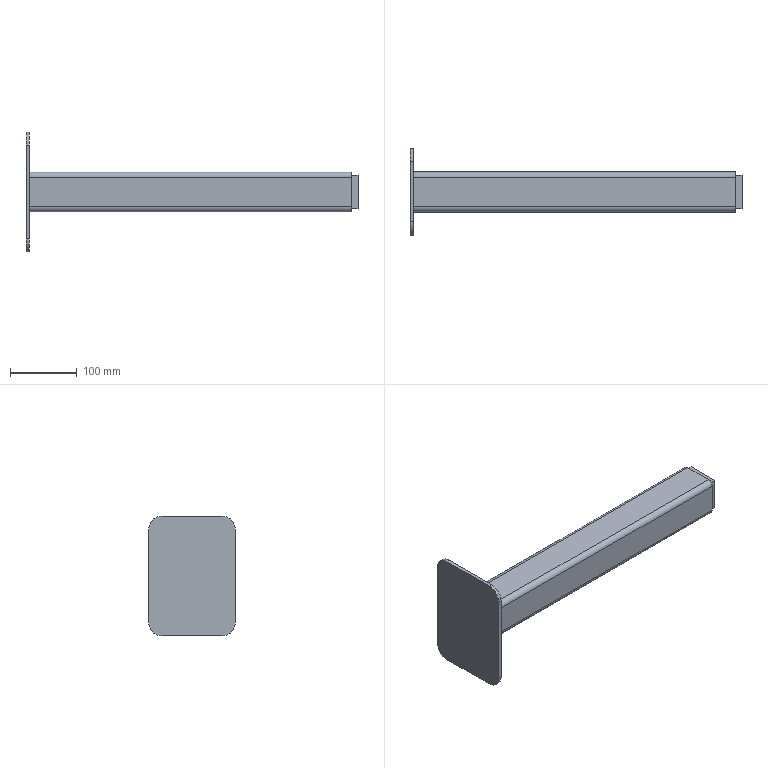Part | SolidWorks | features ICE 2, HoleWzd 1, WeldMemberFeat 1, WeldmentFeature 1 | 3 solids | 36 faces | box 498.5 x 130 x 180 mm | volume 585064 mm3 | plane 22 | cylinder 14 | commonest cylinder face diameters 8 x4 16 x4 40 x4 17.5 x2
STEP:
#1=CARTESIAN_POINT('',(0.,30.,22.));
#2=VERTEX_POINT('',#1);
#3=CARTESIAN_POINT('',(0.,22.,30.));
#4=VERTEX_POINT('',#3);
#5=CARTESIAN_POINT('',(0.,22.,22.));
#6=DIRECTION('',(1.,0.,0.));
#7=DIRECTION('',(0.,0.,-1.));
#8=AXIS2_PLACEMENT_3D('',#5,#6,#7);
#9=CIRCLE('',#8,8.);
#10=EDGE_CURVE('',#2,#4,#9,.T.);
#11=ORIENTED_EDGE('',*,*,#10,.T.);
#12=CARTESIAN_POINT('',(483.5,22.,30.));
#13=VERTEX_POINT('',#12);
#14=CARTESIAN_POINT('',(483.5,22.,30.));
#15=DIRECTION('',(-1.,0.,0.));
#16=VECTOR('',#15,1000.);
#17=LINE('',#14,#16);
#18=EDGE_CURVE('',#13,#4,#17,.T.);
#19=ORIENTED_EDGE('',*,*,#18,.F.);
#20=CARTESIAN_POINT('',(483.5,30.,22.));
#21=VERTEX_POINT('',#20);
#22=CARTESIAN_POINT('',(483.5,22.,22.));
#23=DIRECTION('',(1.,0.,0.));
#24=DIRECTION('',(0.,0.,-1.));
#25=AXIS2_PLACEMENT_3D('',#22,#23,#24);
#26=CIRCLE('',#25,8.);
#27=EDGE_CURVE('',#21,#13,#26,.T.);
#28=ORIENTED_EDGE('',*,*,#27,.F.);
#29=CARTESIAN_POINT('',(483.5,30.,22.));
#30=DIRECTION('',(-1.,0.,0.));
#31=VECTOR('',#30,1000.);
#32=LINE('',#29,#31);
#33=EDGE_CURVE('',#21,#2,#32,.T.);
#34=ORIENTED_EDGE('',*,*,#33,.T.);
#35=EDGE_LOOP('',(#11,#19,#28,#34));
#36=FACE_OUTER_BOUND('',#35,.T.);
#37=CARTESIAN_POINT('',(483.5,22.,22.));
#38=DIRECTION('',(-1.,0.,0.));
#39=DIRECTION('',(0.,0.,1.));
#40=AXIS2_PLACEMENT_3D('',#37,#38,#39);
#41=CYLINDRICAL_SURFACE('',#40,8.);
#42=ADVANCED_FACE('',(#36),#41,.T.);
#43=CARTESIAN_POINT('',(0.,-22.,30.));
#44=VERTEX_POINT('',#43);
#45=CARTESIAN_POINT('',(0.,22.,30.));
#46=DIRECTION('',(0.,-1.,0.));
#47=VECTOR('',#46,1000.);
#48=LINE('',#45,#47);
#49=EDGE_CURVE('',#4,#44,#48,.T.);
#50=ORIENTED_EDGE('',*,*,#49,.T.);
#51=CARTESIAN_POINT('',(483.5,-22.,30.));
#52=VERTEX_POINT('',#51);
#53=CARTESIAN_POINT('',(483.5,-22.,30.));
#54=DIRECTION('',(-1.,0.,0.));
#55=VECTOR('',#54,1000.);
#56=LINE('',#53,#55);
#57=EDGE_CURVE('',#52,#44,#56,.T.);
#58=ORIENTED_EDGE('',*,*,#57,.F.);
#59=CARTESIAN_POINT('',(483.5,22.,30.));
#60=DIRECTION('',(0.,-1.,0.));
#61=VECTOR('',#60,1000.);
#62=LINE('',#59,#61);
#63=EDGE_CURVE('',#13,#52,#62,.T.);
#64=ORIENTED_EDGE('',*,*,#63,.F.);
#65=ORIENTED_EDGE('',*,*,#18,.T.);
#66=EDGE_LOOP('',(#50,#58,#64,#65));
#67=FACE_OUTER_BOUND('',#66,.T.);
#68=CARTESIAN_POINT('',(483.5,22.,30.));
#69=DIRECTION('',(0.,0.,-1.));
#70=DIRECTION('',(-1.,0.,0.));
#71=AXIS2_PLACEMENT_3D('',#68,#69,#70);
#72=PLANE('',#71);
#73=ADVANCED_FACE('',(#67),#72,.F.);
#74=CARTESIAN_POINT('',(0.,-30.,22.));
#75=VERTEX_POINT('',#74);
#76=CARTESIAN_POINT('',(0.,-22.,22.));
#77=DIRECTION('',(1.,0.,0.));
#78=DIRECTION('',(0.,0.,-1.));
#79=AXIS2_PLACEMENT_3D('',#76,#77,#78);
#80=CIRCLE('',#79,8.);
#81=EDGE_CURVE('',#44,#75,#80,.T.);
#82=ORIENTED_EDGE('',*,*,#81,.T.);
#83=CARTESIAN_POINT('',(483.5,-30.,22.));
#84=VERTEX_POINT('',#83);
#85=CARTESIAN_POINT('',(483.5,-30.,22.));
#86=DIRECTION('',(-1.,0.,0.));
#87=VECTOR('',#86,1000.);
#88=LINE('',#85,#87);
#89=EDGE_CURVE('',#84,#75,#88,.T.);
#90=ORIENTED_EDGE('',*,*,#89,.F.);
#91=CARTESIAN_POINT('',(483.5,-22.,22.));
#92=DIRECTION('',(1.,0.,0.));
#93=DIRECTION('',(0.,0.,-1.));
#94=AXIS2_PLACEMENT_3D('',#91,#92,#93);
#95=CIRCLE('',#94,8.);
#96=EDGE_CURVE('',#52,#84,#95,.T.);
#97=ORIENTED_EDGE('',*,*,#96,.F.);
#98=ORIENTED_EDGE('',*,*,#57,.T.);
#99=EDGE_LOOP('',(#82,#90,#97,#98));
#100=FACE_OUTER_BOUND('',#99,.T.);
#101=CARTESIAN_POINT('',(483.5,-22.,22.));
#102=DIRECTION('',(-1.,0.,0.));
#103=DIRECTION('',(0.,0.,1.));
#104=AXIS2_PLACEMENT_3D('',#101,#102,#103);
#105=CYLINDRICAL_SURFACE('',#104,8.);
#106=ADVANCED_FACE('',(#100),#105,.T.);
#107=CARTESIAN_POINT('',(0.,-30.,-22.));
#108=VERTEX_POINT('',#107);
#109=CARTESIAN_POINT('',(0.,-30.,-22.));
#110=DIRECTION('',(0.,0.,-1.));
#111=VECTOR('',#110,1000.);
#112=LINE('',#109,#111);
#113=EDGE_CURVE('',#75,#108,#112,.T.);
#114=ORIENTED_EDGE('',*,*,#113,.T.);
#115=CARTESIAN_POINT('',(483.5,-30.,-22.));
#116=VERTEX_POINT('',#115);
#117=CARTESIAN_POINT('',(483.5,-30.,-22.));
#118=DIRECTION('',(-1.,0.,0.));
#119=VECTOR('',#118,1000.);
#120=LINE('',#117,#119);
#121=EDGE_CURVE('',#116,#108,#120,.T.);
#122=ORIENTED_EDGE('',*,*,#121,.F.);
#123=CARTESIAN_POINT('',(483.5,-30.,-22.));
#124=DIRECTION('',(0.,0.,-1.));
#125=VECTOR('',#124,1000.);
#126=LINE('',#123,#125);
#127=EDGE_CURVE('',#84,#116,#126,.T.);
#128=ORIENTED_EDGE('',*,*,#127,.F.);
#129=ORIENTED_EDGE('',*,*,#89,.T.);
#130=EDGE_LOOP('',(#114,#122,#128,#129));
#131=FACE_OUTER_BOUND('',#130,.T.);
#132=CARTESIAN_POINT('',(483.5,-30.,-22.));
#133=DIRECTION('',(0.,1.,0.));
#134=DIRECTION('',(0.,0.,1.));
#135=AXIS2_PLACEMENT_3D('',#132,#133,#134);
#136=PLANE('',#135);
#137=ADVANCED_FACE('',(#131),#136,.F.);
#138=CARTESIAN_POINT('',(0.,-22.,-30.));
#139=VERTEX_POINT('',#138);
#140=CARTESIAN_POINT('',(0.,-22.,-22.));
#141=DIRECTION('',(1.,0.,0.));
#142=DIRECTION('',(0.,0.,-1.));
#143=AXIS2_PLACEMENT_3D('',#140,#141,#142);
#144=CIRCLE('',#143,8.);
#145=EDGE_CURVE('',#108,#139,#144,.T.);
#146=ORIENTED_EDGE('',*,*,#145,.T.);
#147=CARTESIAN_POINT('',(483.5,-22.,-30.));
#148=VERTEX_POINT('',#147);
#149=CARTESIAN_POINT('',(483.5,-22.,-30.));
#150=DIRECTION('',(-1.,0.,0.));
#151=VECTOR('',#150,1000.);
#152=LINE('',#149,#151);
#153=EDGE_CURVE('',#148,#139,#152,.T.);
#154=ORIENTED_EDGE('',*,*,#153,.F.);
#155=CARTESIAN_POINT('',(483.5,-22.,-22.));
#156=DIRECTION('',(1.,0.,0.));
#157=DIRECTION('',(0.,0.,-1.));
#158=AXIS2_PLACEMENT_3D('',#155,#156,#157);
#159=CIRCLE('',#158,8.);
#160=EDGE_CURVE('',#116,#148,#159,.T.);
#161=ORIENTED_EDGE('',*,*,#160,.F.);
#162=ORIENTED_EDGE('',*,*,#121,.T.);
#163=EDGE_LOOP('',(#146,#154,#161,#162));
#164=FACE_OUTER_BOUND('',#163,.T.);
#165=CARTESIAN_POINT('',(483.5,-22.,-22.));
#166=DIRECTION('',(-1.,0.,0.));
#167=DIRECTION('',(0.,0.,1.));
#168=AXIS2_PLACEMENT_3D('',#165,#166,#167);
#169=CYLINDRICAL_SURFACE('',#168,8.);
#170=ADVANCED_FACE('',(#164),#169,.T.);
#171=CARTESIAN_POINT('',(0.,22.,-30.));
#172=VERTEX_POINT('',#171);
#173=CARTESIAN_POINT('',(0.,-22.,-30.));
#174=DIRECTION('',(0.,1.,0.));
#175=VECTOR('',#174,1000.);
#176=LINE('',#173,#175);
#177=EDGE_CURVE('',#139,#172,#176,.T.);
#178=ORIENTED_EDGE('',*,*,#177,.T.);
#179=CARTESIAN_POINT('',(483.5,22.,-30.));
#180=VERTEX_POINT('',#179);
#181=CARTESIAN_POINT('',(483.5,22.,-30.));
#182=DIRECTION('',(-1.,0.,0.));
#183=VECTOR('',#182,1000.);
#184=LINE('',#181,#183);
#185=EDGE_CURVE('',#180,#172,#184,.T.);
#186=ORIENTED_EDGE('',*,*,#185,.F.);
#187=CARTESIAN_POINT('',(483.5,-22.,-30.));
#188=DIRECTION('',(0.,1.,0.));
#189=VECTOR('',#188,1000.);
#190=LINE('',#187,#189);
#191=EDGE_CURVE('',#148,#180,#190,.T.);
#192=ORIENTED_EDGE('',*,*,#191,.F.);
#193=ORIENTED_EDGE('',*,*,#153,.T.);
#194=EDGE_LOOP('',(#178,#186,#192,#193));
#195=FACE_OUTER_BOUND('',#194,.T.);
#196=CARTESIAN_POINT('',(483.5,-22.,-30.));
#197=DIRECTION('',(0.,0.,1.));
#198=DIRECTION('',(1.,0.,0.));
#199=AXIS2_PLACEMENT_3D('',#196,#197,#198);
#200=PLANE('',#199);
#201=ADVANCED_FACE('',(#195),#200,.F.);
#202=CARTESIAN_POINT('',(0.,30.,-22.));
#203=VERTEX_POINT('',#202);
#204=CARTESIAN_POINT('',(0.,22.,-22.));
#205=DIRECTION('',(1.,0.,0.));
#206=DIRECTION('',(0.,0.,-1.));
#207=AXIS2_PLACEMENT_3D('',#204,#205,#206);
#208=CIRCLE('',#207,8.);
#209=EDGE_CURVE('',#172,#203,#208,.T.);
#210=ORIENTED_EDGE('',*,*,#209,.T.);
#211=CARTESIAN_POINT('',(483.5,30.,-22.));
#212=VERTEX_POINT('',#211);
#213=CARTESIAN_POINT('',(483.5,30.,-22.));
#214=DIRECTION('',(-1.,0.,0.));
#215=VECTOR('',#214,1000.);
#216=LINE('',#213,#215);
#217=EDGE_CURVE('',#212,#203,#216,.T.);
#218=ORIENTED_EDGE('',*,*,#217,.F.);
#219=CARTESIAN_POINT('',(483.5,22.,-22.));
#220=DIRECTION('',(1.,0.,0.));
#221=DIRECTION('',(0.,0.,-1.));
#222=AXIS2_PLACEMENT_3D('',#219,#220,#221);
#223=CIRCLE('',#222,8.);
#224=EDGE_CURVE('',#180,#212,#223,.T.);
#225=ORIENTED_EDGE('',*,*,#224,.F.);
#226=ORIENTED_EDGE('',*,*,#185,.T.);
#227=EDGE_LOOP('',(#210,#218,#225,#226));
#228=FACE_OUTER_BOUND('',#227,.T.);
#229=CARTESIAN_POINT('',(483.5,22.,-22.));
#230=DIRECTION('',(-1.,0.,0.));
#231=DIRECTION('',(0.,0.,1.));
#232=AXIS2_PLACEMENT_3D('',#229,#230,#231);
#233=CYLINDRICAL_SURFACE('',#232,8.);
#234=ADVANCED_FACE('',(#228),#233,.T.);
#235=CARTESIAN_POINT('',(0.,-22.,26.));
#236=VERTEX_POINT('',#235);
#237=CARTESIAN_POINT('',(0.,-26.,22.));
#238=VERTEX_POINT('',#237);
#239=CARTESIAN_POINT('',(0.,-22.,22.));
#240=DIRECTION('',(1.,0.,0.));
#241=DIRECTION('',(0.,0.,-1.));
#242=AXIS2_PLACEMENT_3D('',#239,#240,#241);
#243=CIRCLE('',#242,4.);
#244=EDGE_CURVE('',#236,#238,#243,.T.);
#245=ORIENTED_EDGE('',*,*,#244,.F.);
#246=CARTESIAN_POINT('',(483.5,-22.,26.));
#247=VERTEX_POINT('',#246);
#248=CARTESIAN_POINT('',(483.5,-22.,26.));
#249=DIRECTION('',(-1.,0.,0.));
#250=VECTOR('',#249,1000.);
#251=LINE('',#248,#250);
#252=EDGE_CURVE('',#247,#236,#251,.T.);
#253=ORIENTED_EDGE('',*,*,#252,.F.);
#254=CARTESIAN_POINT('',(483.5,-26.,22.));
#255=VERTEX_POINT('',#254);
#256=CARTESIAN_POINT('',(483.5,-22.,22.));
#257=DIRECTION('',(1.,0.,0.));
#258=DIRECTION('',(0.,0.,-1.));
#259=AXIS2_PLACEMENT_3D('',#256,#257,#258);
#260=CIRCLE('',#259,4.);
#261=EDGE_CURVE('',#247,#255,#260,.T.);
#262=ORIENTED_EDGE('',*,*,#261,.T.);
#263=CARTESIAN_POINT('',(483.5,-26.,22.));
#264=DIRECTION('',(-1.,0.,0.));
#265=VECTOR('',#264,1000.);
#266=LINE('',#263,#265);
#267=EDGE_CURVE('',#255,#238,#266,.T.);
#268=ORIENTED_EDGE('',*,*,#267,.T.);
#269=EDGE_LOOP('',(#245,#253,#262,#268));
#270=FACE_OUTER_BOUND('',#269,.T.);
#271=CARTESIAN_POINT('',(483.5,-22.,22.));
#272=DIRECTION('',(-1.,0.,0.));
#273=DIRECTION('',(0.,0.,1.));
#274=AXIS2_PLACEMENT_3D('',#271,#272,#273);
#275=CYLINDRICAL_SURFACE('',#274,4.);
#276=ADVANCED_FACE('',(#270),#275,.F.);
#277=CARTESIAN_POINT('',(0.,22.,26.));
#278=VERTEX_POINT('',#277);
#279=CARTESIAN_POINT('',(0.,22.,26.));
#280=DIRECTION('',(0.,-1.,0.));
#281=VECTOR('',#280,1000.);
#282=LINE('',#279,#281);
#283=EDGE_CURVE('',#278,#236,#282,.T.);
#284=ORIENTED_EDGE('',*,*,#283,.F.);
#285=CARTESIAN_POINT('',(483.5,22.,26.));
#286=VERTEX_POINT('',#285);
#287=CARTESIAN_POINT('',(483.5,22.,26.));
#288=DIRECTION('',(-1.,0.,0.));
#289=VECTOR('',#288,1000.);
#290=LINE('',#287,#289);
#291=EDGE_CURVE('',#286,#278,#290,.T.);
#292=ORIENTED_EDGE('',*,*,#291,.F.);
#293=CARTESIAN_POINT('',(483.5,22.,26.));
#294=DIRECTION('',(0.,-1.,0.));
#295=VECTOR('',#294,1000.);
#296=LINE('',#293,#295);
#297=EDGE_CURVE('',#286,#247,#296,.T.);
#298=ORIENTED_EDGE('',*,*,#297,.T.);
#299=ORIENTED_EDGE('',*,*,#252,.T.);
#300=EDGE_LOOP('',(#284,#292,#298,#299));
#301=FACE_OUTER_BOUND('',#300,.T.);
#302=CARTESIAN_POINT('',(483.5,22.,26.));
#303=DIRECTION('',(0.,0.,-1.));
#304=DIRECTION('',(-1.,0.,0.));
#305=AXIS2_PLACEMENT_3D('',#302,#303,#304);
#306=PLANE('',#305);
#307=ADVANCED_FACE('',(#301),#306,.T.);
#308=CARTESIAN_POINT('',(0.,26.,22.));
#309=VERTEX_POINT('',#308);
#310=CARTESIAN_POINT('',(0.,22.,22.));
#311=DIRECTION('',(1.,0.,0.));
#312=DIRECTION('',(0.,0.,-1.));
#313=AXIS2_PLACEMENT_3D('',#310,#311,#312);
#314=CIRCLE('',#313,4.);
#315=EDGE_CURVE('',#309,#278,#314,.T.);
#316=ORIENTED_EDGE('',*,*,#315,.F.);
#317=CARTESIAN_POINT('',(483.5,26.,22.));
#318=VERTEX_POINT('',#317);
#319=CARTESIAN_POINT('',(483.5,26.,22.));
#320=DIRECTION('',(-1.,0.,0.));
#321=VECTOR('',#320,1000.);
#322=LINE('',#319,#321);
#323=EDGE_CURVE('',#318,#309,#322,.T.);
#324=ORIENTED_EDGE('',*,*,#323,.F.);
#325=CARTESIAN_POINT('',(483.5,22.,22.));
#326=DIRECTION('',(1.,0.,0.));
#327=DIRECTION('',(0.,0.,-1.));
#328=AXIS2_PLACEMENT_3D('',#325,#326,#327);
#329=CIRCLE('',#328,4.);
#330=EDGE_CURVE('',#318,#286,#329,.T.);
#331=ORIENTED_EDGE('',*,*,#330,.T.);
#332=ORIENTED_EDGE('',*,*,#291,.T.);
#333=EDGE_LOOP('',(#316,#324,#331,#332));
#334=FACE_OUTER_BOUND('',#333,.T.);
#335=CARTESIAN_POINT('',(483.5,22.,22.));
#336=DIRECTION('',(-1.,0.,0.));
#337=DIRECTION('',(0.,0.,1.));
#338=AXIS2_PLACEMENT_3D('',#335,#336,#337);
#339=CYLINDRICAL_SURFACE('',#338,4.);
#340=ADVANCED_FACE('',(#334),#339,.F.);
#341=CARTESIAN_POINT('',(0.,26.,-22.));
#342=VERTEX_POINT('',#341);
#343=CARTESIAN_POINT('',(0.,26.,22.));
#344=DIRECTION('',(0.,0.,1.));
#345=VECTOR('',#344,1000.);
#346=LINE('',#343,#345);
#347=EDGE_CURVE('',#342,#309,#346,.T.);
#348=ORIENTED_EDGE('',*,*,#347,.F.);
#349=CARTESIAN_POINT('',(483.5,26.,-22.));
#350=VERTEX_POINT('',#349);
#351=CARTESIAN_POINT('',(483.5,26.,-22.));
#352=DIRECTION('',(-1.,0.,0.));
#353=VECTOR('',#352,1000.);
#354=LINE('',#351,#353);
#355=EDGE_CURVE('',#350,#342,#354,.T.);
#356=ORIENTED_EDGE('',*,*,#355,.F.);
#357=CARTESIAN_POINT('',(483.5,26.,22.));
#358=DIRECTION('',(0.,0.,1.));
#359=VECTOR('',#358,1000.);
#360=LINE('',#357,#359);
#361=EDGE_CURVE('',#350,#318,#360,.T.);
#362=ORIENTED_EDGE('',*,*,#361,.T.);
#363=ORIENTED_EDGE('',*,*,#323,.T.);
#364=EDGE_LOOP('',(#348,#356,#362,#363));
#365=FACE_OUTER_BOUND('',#364,.T.);
#366=CARTESIAN_POINT('',(483.5,26.,22.));
#367=DIRECTION('',(0.,-1.,0.));
#368=DIRECTION('',(0.,0.,-1.));
#369=AXIS2_PLACEMENT_3D('',#366,#367,#368);
#370=PLANE('',#369);
#371=ADVANCED_FACE('',(#365),#370,.T.);
#372=CARTESIAN_POINT('',(0.,22.,-26.));
#373=VERTEX_POINT('',#372);
#374=CARTESIAN_POINT('',(0.,22.,-22.));
#375=DIRECTION('',(1.,0.,0.));
#376=DIRECTION('',(0.,0.,-1.));
#377=AXIS2_PLACEMENT_3D('',#374,#375,#376);
#378=CIRCLE('',#377,4.);
#379=EDGE_CURVE('',#373,#342,#378,.T.);
#380=ORIENTED_EDGE('',*,*,#379,.F.);
#381=CARTESIAN_POINT('',(483.5,22.,-26.));
#382=VERTEX_POINT('',#381);
#383=CARTESIAN_POINT('',(483.5,22.,-26.));
#384=DIRECTION('',(-1.,0.,0.));
#385=VECTOR('',#384,1000.);
#386=LINE('',#383,#385);
#387=EDGE_CURVE('',#382,#373,#386,.T.);
#388=ORIENTED_EDGE('',*,*,#387,.F.);
#389=CARTESIAN_POINT('',(483.5,22.,-22.));
#390=DIRECTION('',(1.,0.,0.));
#391=DIRECTION('',(0.,0.,-1.));
#392=AXIS2_PLACEMENT_3D('',#389,#390,#391);
#393=CIRCLE('',#392,4.);
#394=EDGE_CURVE('',#382,#350,#393,.T.);
#395=ORIENTED_EDGE('',*,*,#394,.T.);
#396=ORIENTED_EDGE('',*,*,#355,.T.);
#397=EDGE_LOOP('',(#380,#388,#395,#396));
#398=FACE_OUTER_BOUND('',#397,.T.);
#399=CARTESIAN_POINT('',(483.5,22.,-22.));
#400=DIRECTION('',(-1.,0.,0.));
#401=DIRECTION('',(0.,0.,1.));
#402=AXIS2_PLACEMENT_3D('',#399,#400,#401);
#403=CYLINDRICAL_SURFACE('',#402,4.);
#404=ADVANCED_FACE('',(#398),#403,.F.);
#405=CARTESIAN_POINT('',(0.,-22.,-26.));
#406=VERTEX_POINT('',#405);
#407=CARTESIAN_POINT('',(0.,-22.,-26.));
#408=DIRECTION('',(0.,1.,0.));
#409=VECTOR('',#408,1000.);
#410=LINE('',#407,#409);
#411=EDGE_CURVE('',#406,#373,#410,.T.);
#412=ORIENTED_EDGE('',*,*,#411,.F.);
#413=CARTESIAN_POINT('',(483.5,-22.,-26.));
#414=VERTEX_POINT('',#413);
#415=CARTESIAN_POINT('',(483.5,-22.,-26.));
#416=DIRECTION('',(-1.,0.,0.));
#417=VECTOR('',#416,1000.);
#418=LINE('',#415,#417);
#419=EDGE_CURVE('',#414,#406,#418,.T.);
#420=ORIENTED_EDGE('',*,*,#419,.F.);
#421=CARTESIAN_POINT('',(483.5,-22.,-26.));
#422=DIRECTION('',(0.,1.,0.));
#423=VECTOR('',#422,1000.);
#424=LINE('',#421,#423);
#425=EDGE_CURVE('',#414,#382,#424,.T.);
#426=ORIENTED_EDGE('',*,*,#425,.T.);
#427=ORIENTED_EDGE('',*,*,#387,.T.);
#428=EDGE_LOOP('',(#412,#420,#426,#427));
#429=FACE_OUTER_BOUND('',#428,.T.);
#430=CARTESIAN_POINT('',(483.5,-22.,-26.));
#431=DIRECTION('',(0.,0.,1.));
#432=DIRECTION('',(1.,0.,0.));
#433=AXIS2_PLACEMENT_3D('',#430,#431,#432);
#434=PLANE('',#433);
#435=ADVANCED_FACE('',(#429),#434,.T.);
#436=CARTESIAN_POINT('',(0.,-26.,-22.));
#437=VERTEX_POINT('',#436);
#438=CARTESIAN_POINT('',(0.,-22.,-22.));
#439=DIRECTION('',(1.,0.,0.));
#440=DIRECTION('',(0.,0.,-1.));
#441=AXIS2_PLACEMENT_3D('',#438,#439,#440);
#442=CIRCLE('',#441,4.);
#443=EDGE_CURVE('',#437,#406,#442,.T.);
#444=ORIENTED_EDGE('',*,*,#443,.F.);
#445=CARTESIAN_POINT('',(483.5,-26.,-22.));
#446=VERTEX_POINT('',#445);
#447=CARTESIAN_POINT('',(483.5,-26.,-22.));
#448=DIRECTION('',(-1.,0.,0.));
#449=VECTOR('',#448,1000.);
#450=LINE('',#447,#449);
#451=EDGE_CURVE('',#446,#437,#450,.T.);
#452=ORIENTED_EDGE('',*,*,#451,.F.);
#453=CARTESIAN_POINT('',(483.5,-22.,-22.));
#454=DIRECTION('',(1.,0.,0.));
#455=DIRECTION('',(0.,0.,-1.));
#456=AXIS2_PLACEMENT_3D('',#453,#454,#455);
#457=CIRCLE('',#456,4.);
#458=EDGE_CURVE('',#446,#414,#457,.T.);
#459=ORIENTED_EDGE('',*,*,#458,.T.);
#460=ORIENTED_EDGE('',*,*,#419,.T.);
#461=EDGE_LOOP('',(#444,#452,#459,#460));
#462=FACE_OUTER_BOUND('',#461,.T.);
#463=CARTESIAN_POINT('',(483.5,-22.,-22.));
#464=DIRECTION('',(-1.,0.,0.));
#465=DIRECTION('',(0.,0.,1.));
#466=AXIS2_PLACEMENT_3D('',#463,#464,#465);
#467=CYLINDRICAL_SURFACE('',#466,4.);
#468=ADVANCED_FACE('',(#462),#467,.F.);
#469=CARTESIAN_POINT('',(0.,-26.,-22.));
#470=DIRECTION('',(0.,0.,-1.));
#471=VECTOR('',#470,1000.);
#472=LINE('',#469,#471);
#473=EDGE_CURVE('',#238,#437,#472,.T.);
#474=ORIENTED_EDGE('',*,*,#473,.F.);
#475=ORIENTED_EDGE('',*,*,#267,.F.);
#476=CARTESIAN_POINT('',(483.5,-26.,-22.));
#477=DIRECTION('',(0.,0.,-1.));
#478=VECTOR('',#477,1000.);
#479=LINE('',#476,#478);
#480=EDGE_CURVE('',#255,#446,#479,.T.);
#481=ORIENTED_EDGE('',*,*,#480,.T.);
#482=ORIENTED_EDGE('',*,*,#451,.T.);
#483=EDGE_LOOP('',(#474,#475,#481,#482));
#484=FACE_OUTER_BOUND('',#483,.T.);
#485=CARTESIAN_POINT('',(483.5,-26.,-22.));
#486=DIRECTION('',(0.,1.,0.));
#487=DIRECTION('',(0.,0.,1.));
#488=AXIS2_PLACEMENT_3D('',#485,#486,#487);
#489=PLANE('',#488);
#490=ADVANCED_FACE('',(#484),#489,.T.);
#491=CARTESIAN_POINT('',(0.,30.,22.));
#492=DIRECTION('',(0.,0.,1.));
#493=VECTOR('',#492,1000.);
#494=LINE('',#491,#493);
#495=EDGE_CURVE('',#203,#2,#494,.T.);
#496=ORIENTED_EDGE('',*,*,#495,.T.);
#497=ORIENTED_EDGE('',*,*,#33,.F.);
#498=CARTESIAN_POINT('',(483.5,30.,22.));
#499=DIRECTION('',(0.,0.,1.));
#500=VECTOR('',#499,1000.);
#501=LINE('',#498,#500);
#502=EDGE_CURVE('',#212,#21,#501,.T.);
#503=ORIENTED_EDGE('',*,*,#502,.F.);
#504=ORIENTED_EDGE('',*,*,#217,.T.);
#505=EDGE_LOOP('',(#496,#497,#503,#504));
#506=FACE_OUTER_BOUND('',#505,.T.);
#507=CARTESIAN_POINT('',(483.5,30.,22.));
#508=DIRECTION('',(0.,-1.,0.));
#509=DIRECTION('',(0.,0.,-1.));
#510=AXIS2_PLACEMENT_3D('',#507,#508,#509);
#511=PLANE('',#510);
#512=ADVANCED_FACE('',(#506),#511,.F.);
#513=ORIENTED_EDGE('',*,*,#261,.F.);
#514=ORIENTED_EDGE('',*,*,#297,.F.);
#515=ORIENTED_EDGE('',*,*,#330,.F.);
#516=ORIENTED_EDGE('',*,*,#361,.F.);
#517=ORIENTED_EDGE('',*,*,#394,.F.);
#518=ORIENTED_EDGE('',*,*,#425,.F.);
#519=ORIENTED_EDGE('',*,*,#458,.F.);
#520=ORIENTED_EDGE('',*,*,#480,.F.);
#521=EDGE_LOOP('',(#513,#514,#515,#516,#517,#518,#519,#520));
#522=FACE_BOUND('',#521,.T.);
#523=ORIENTED_EDGE('',*,*,#27,.T.);
#524=ORIENTED_EDGE('',*,*,#63,.T.);
#525=ORIENTED_EDGE('',*,*,#96,.T.);
#526=ORIENTED_EDGE('',*,*,#127,.T.);
#527=ORIENTED_EDGE('',*,*,#160,.T.);
#528=ORIENTED_EDGE('',*,*,#191,.T.);
#529=ORIENTED_EDGE('',*,*,#224,.T.);
#530=ORIENTED_EDGE('',*,*,#502,.T.);
#531=EDGE_LOOP('',(#523,#524,#525,#526,#527,#528,#529,#530));
#532=FACE_OUTER_BOUND('',#531,.T.);
#533=CARTESIAN_POINT('',(483.5,22.,22.));
#534=DIRECTION('',(1.,0.,0.));
#535=DIRECTION('',(0.,0.,-1.));
#536=AXIS2_PLACEMENT_3D('',#533,#534,#535);
#537=PLANE('',#536);
#538=ADVANCED_FACE('',(#522,#532),#537,.T.);
#539=ORIENTED_EDGE('',*,*,#244,.T.);
#540=ORIENTED_EDGE('',*,*,#473,.T.);
#541=ORIENTED_EDGE('',*,*,#443,.T.);
#542=ORIENTED_EDGE('',*,*,#411,.T.);
#543=ORIENTED_EDGE('',*,*,#379,.T.);
#544=ORIENTED_EDGE('',*,*,#347,.T.);
#545=ORIENTED_EDGE('',*,*,#315,.T.);
#546=ORIENTED_EDGE('',*,*,#283,.T.);
#547=EDGE_LOOP('',(#539,#540,#541,#542,#543,#544,#545,#546));
#548=FACE_BOUND('',#547,.T.);
#549=ORIENTED_EDGE('',*,*,#10,.F.);
#550=ORIENTED_EDGE('',*,*,#495,.F.);
#551=ORIENTED_EDGE('',*,*,#209,.F.);
#552=ORIENTED_EDGE('',*,*,#177,.F.);
#553=ORIENTED_EDGE('',*,*,#145,.F.);
#554=ORIENTED_EDGE('',*,*,#113,.F.);
#555=ORIENTED_EDGE('',*,*,#81,.F.);
#556=ORIENTED_EDGE('',*,*,#49,.F.);
#557=EDGE_LOOP('',(#549,#550,#551,#552,#553,#554,#555,#556));
#558=FACE_OUTER_BOUND('',#557,.T.);
#559=CARTESIAN_POINT('',(0.,22.,22.));
#560=DIRECTION('',(1.,0.,0.));
#561=DIRECTION('',(0.,0.,-1.));
#562=AXIS2_PLACEMENT_3D('',#559,#560,#561);
#563=PLANE('',#562);
#564=ADVANCED_FACE('',(#548,#558),#563,.F.);
#565=CLOSED_SHELL('',(#42,#73,#106,#137,#170,#201,#234,#276,#307,#340,#371,#404,#435,#468,#490,#512,#538,#564));
#566=MANIFOLD_SOLID_BREP('',#565);
#567=CARTESIAN_POINT('',(0.,45.,90.));
#568=VERTEX_POINT('',#567);
#569=CARTESIAN_POINT('',(0.,65.,70.));
#570=VERTEX_POINT('',#569);
#571=CARTESIAN_POINT('',(0.,45.,70.));
#572=DIRECTION('',(-1.,0.,0.));
#573=DIRECTION('',(0.,0.,-1.));
#574=AXIS2_PLACEMENT_3D('',#571,#572,#573);
#575=CIRCLE('',#574,20.);
#576=EDGE_CURVE('',#568,#570,#575,.T.);
#577=ORIENTED_EDGE('',*,*,#576,.T.);
#578=CARTESIAN_POINT('',(-5.,65.,70.));
#579=VERTEX_POINT('',#578);
#580=CARTESIAN_POINT('',(-5.,65.,70.));
#581=DIRECTION('',(1.,0.,0.));
#582=VECTOR('',#581,1000.);
#583=LINE('',#580,#582);
#584=EDGE_CURVE('',#579,#570,#583,.T.);
#585=ORIENTED_EDGE('',*,*,#584,.F.);
#586=CARTESIAN_POINT('',(-5.,45.,90.));
#587=VERTEX_POINT('',#586);
#588=CARTESIAN_POINT('',(-5.,45.,70.));
#589=DIRECTION('',(-1.,0.,0.));
#590=DIRECTION('',(0.,0.,-1.));
#591=AXIS2_PLACEMENT_3D('',#588,#589,#590);
#592=CIRCLE('',#591,20.);
#593=EDGE_CURVE('',#587,#579,#592,.T.);
#594=ORIENTED_EDGE('',*,*,#593,.F.);
#595=CARTESIAN_POINT('',(-5.,45.,90.));
#596=DIRECTION('',(1.,0.,0.));
#597=VECTOR('',#596,1000.);
#598=LINE('',#595,#597);
#599=EDGE_CURVE('',#587,#568,#598,.T.);
#600=ORIENTED_EDGE('',*,*,#599,.T.);
#601=EDGE_LOOP('',(#577,#585,#594,#600));
#602=FACE_OUTER_BOUND('',#601,.T.);
#603=CARTESIAN_POINT('',(-5.,45.,70.));
#604=DIRECTION('',(1.,0.,0.));
#605=DIRECTION('',(0.,0.,-1.));
#606=AXIS2_PLACEMENT_3D('',#603,#604,#605);
#607=CYLINDRICAL_SURFACE('',#606,20.);
#608=ADVANCED_FACE('',(#602),#607,.T.);
#609=CARTESIAN_POINT('',(0.,65.,-70.));
#610=VERTEX_POINT('',#609);
#611=CARTESIAN_POINT('',(0.,65.,-70.));
#612=DIRECTION('',(0.,0.,-1.));
#613=VECTOR('',#612,1000.);
#614=LINE('',#611,#613);
#615=EDGE_CURVE('',#570,#610,#614,.T.);
#616=ORIENTED_EDGE('',*,*,#615,.T.);
#617=CARTESIAN_POINT('',(-5.,65.,-70.));
#618=VERTEX_POINT('',#617);
#619=CARTESIAN_POINT('',(-5.,65.,-70.));
#620=DIRECTION('',(1.,0.,0.));
#621=VECTOR('',#620,1000.);
#622=LINE('',#619,#621);
#623=EDGE_CURVE('',#618,#610,#622,.T.);
#624=ORIENTED_EDGE('',*,*,#623,.F.);
#625=CARTESIAN_POINT('',(-5.,65.,-70.));
#626=DIRECTION('',(0.,0.,-1.));
#627=VECTOR('',#626,1000.);
#628=LINE('',#625,#627);
#629=EDGE_CURVE('',#579,#618,#628,.T.);
#630=ORIENTED_EDGE('',*,*,#629,.F.);
#631=ORIENTED_EDGE('',*,*,#584,.T.);
#632=EDGE_LOOP('',(#616,#624,#630,#631));
#633=FACE_OUTER_BOUND('',#632,.T.);
#634=CARTESIAN_POINT('',(-5.,65.,-70.));
#635=DIRECTION('',(0.,-1.,0.));
#636=DIRECTION('',(0.,0.,-1.));
#637=AXIS2_PLACEMENT_3D('',#634,#635,#636);
#638=PLANE('',#637);
#639=ADVANCED_FACE('',(#633),#638,.F.);
#640=CARTESIAN_POINT('',(0.,45.,-90.));
#641=VERTEX_POINT('',#640);
#642=CARTESIAN_POINT('',(0.,45.,-70.));
#643=DIRECTION('',(-1.,0.,0.));
#644=DIRECTION('',(0.,0.,1.));
#645=AXIS2_PLACEMENT_3D('',#642,#643,#644);
#646=CIRCLE('',#645,20.);
#647=EDGE_CURVE('',#610,#641,#646,.T.);
#648=ORIENTED_EDGE('',*,*,#647,.T.);
#649=CARTESIAN_POINT('',(-5.,45.,-90.));
#650=VERTEX_POINT('',#649);
#651=CARTESIAN_POINT('',(-5.,45.,-90.));
#652=DIRECTION('',(1.,0.,0.));
#653=VECTOR('',#652,1000.);
#654=LINE('',#651,#653);
#655=EDGE_CURVE('',#650,#641,#654,.T.);
#656=ORIENTED_EDGE('',*,*,#655,.F.);
#657=CARTESIAN_POINT('',(-5.,45.,-70.));
#658=DIRECTION('',(-1.,0.,0.));
#659=DIRECTION('',(0.,0.,1.));
#660=AXIS2_PLACEMENT_3D('',#657,#658,#659);
#661=CIRCLE('',#660,20.);
#662=EDGE_CURVE('',#618,#650,#661,.T.);
#663=ORIENTED_EDGE('',*,*,#662,.F.);
#664=ORIENTED_EDGE('',*,*,#623,.T.);
#665=EDGE_LOOP('',(#648,#656,#663,#664));
#666=FACE_OUTER_BOUND('',#665,.T.);
#667=CARTESIAN_POINT('',(-5.,45.,-70.));
#668=DIRECTION('',(1.,0.,0.));
#669=DIRECTION('',(0.,0.,-1.));
#670=AXIS2_PLACEMENT_3D('',#667,#668,#669);
#671=CYLINDRICAL_SURFACE('',#670,20.);
#672=ADVANCED_FACE('',(#666),#671,.T.);
#673=CARTESIAN_POINT('',(0.,-45.,-90.));
#674=VERTEX_POINT('',#673);
#675=CARTESIAN_POINT('',(0.,45.,-90.));
#676=DIRECTION('',(0.,-1.,0.));
#677=VECTOR('',#676,1000.);
#678=LINE('',#675,#677);
#679=EDGE_CURVE('',#641,#674,#678,.T.);
#680=ORIENTED_EDGE('',*,*,#679,.T.);
#681=CARTESIAN_POINT('',(-5.,-45.,-90.));
#682=VERTEX_POINT('',#681);
#683=CARTESIAN_POINT('',(-5.,-45.,-90.));
#684=DIRECTION('',(1.,0.,0.));
#685=VECTOR('',#684,1000.);
#686=LINE('',#683,#685);
#687=EDGE_CURVE('',#682,#674,#686,.T.);
#688=ORIENTED_EDGE('',*,*,#687,.F.);
#689=CARTESIAN_POINT('',(-5.,45.,-90.));
#690=DIRECTION('',(0.,-1.,0.));
#691=VECTOR('',#690,1000.);
#692=LINE('',#689,#691);
#693=EDGE_CURVE('',#650,#682,#692,.T.);
#694=ORIENTED_EDGE('',*,*,#693,.F.);
#695=ORIENTED_EDGE('',*,*,#655,.T.);
#696=EDGE_LOOP('',(#680,#688,#694,#695));
#697=FACE_OUTER_BOUND('',#696,.T.);
#698=CARTESIAN_POINT('',(-5.,45.,-90.));
#699=DIRECTION('',(0.,0.,1.));
#700=DIRECTION('',(0.,-1.,0.));
#701=AXIS2_PLACEMENT_3D('',#698,#699,#700);
#702=PLANE('',#701);
#703=ADVANCED_FACE('',(#697),#702,.F.);
#704=CARTESIAN_POINT('',(0.,-65.,-70.));
#705=VERTEX_POINT('',#704);
#706=CARTESIAN_POINT('',(0.,-45.,-70.));
#707=DIRECTION('',(-1.,0.,0.));
#708=DIRECTION('',(0.,0.,1.));
#709=AXIS2_PLACEMENT_3D('',#706,#707,#708);
#710=CIRCLE('',#709,20.);
#711=EDGE_CURVE('',#674,#705,#710,.T.);
#712=ORIENTED_EDGE('',*,*,#711,.T.);
#713=CARTESIAN_POINT('',(-5.,-65.,-70.));
#714=VERTEX_POINT('',#713);
#715=CARTESIAN_POINT('',(-5.,-65.,-70.));
#716=DIRECTION('',(1.,0.,0.));
#717=VECTOR('',#716,1000.);
#718=LINE('',#715,#717);
#719=EDGE_CURVE('',#714,#705,#718,.T.);
#720=ORIENTED_EDGE('',*,*,#719,.F.);
#721=CARTESIAN_POINT('',(-5.,-45.,-70.));
#722=DIRECTION('',(-1.,0.,0.));
#723=DIRECTION('',(0.,0.,1.));
#724=AXIS2_PLACEMENT_3D('',#721,#722,#723);
#725=CIRCLE('',#724,20.);
#726=EDGE_CURVE('',#682,#714,#725,.T.);
#727=ORIENTED_EDGE('',*,*,#726,.F.);
#728=ORIENTED_EDGE('',*,*,#687,.T.);
#729=EDGE_LOOP('',(#712,#720,#727,#728));
#730=FACE_OUTER_BOUND('',#729,.T.);
#731=CARTESIAN_POINT('',(-5.,-45.,-70.));
#732=DIRECTION('',(1.,0.,0.));
#733=DIRECTION('',(0.,0.,-1.));
#734=AXIS2_PLACEMENT_3D('',#731,#732,#733);
#735=CYLINDRICAL_SURFACE('',#734,20.);
#736=ADVANCED_FACE('',(#730),#735,.T.);
#737=CARTESIAN_POINT('',(0.,-65.,70.));
#738=VERTEX_POINT('',#737);
#739=CARTESIAN_POINT('',(0.,-65.,-70.));
#740=DIRECTION('',(0.,0.,1.));
#741=VECTOR('',#740,1000.);
#742=LINE('',#739,#741);
#743=EDGE_CURVE('',#705,#738,#742,.T.);
#744=ORIENTED_EDGE('',*,*,#743,.T.);
#745=CARTESIAN_POINT('',(-5.,-65.,70.));
#746=VERTEX_POINT('',#745);
#747=CARTESIAN_POINT('',(-5.,-65.,70.));
#748=DIRECTION('',(1.,0.,0.));
#749=VECTOR('',#748,1000.);
#750=LINE('',#747,#749);
#751=EDGE_CURVE('',#746,#738,#750,.T.);
#752=ORIENTED_EDGE('',*,*,#751,.F.);
#753=CARTESIAN_POINT('',(-5.,-65.,-70.));
#754=DIRECTION('',(0.,0.,1.));
#755=VECTOR('',#754,1000.);
#756=LINE('',#753,#755);
#757=EDGE_CURVE('',#714,#746,#756,.T.);
#758=ORIENTED_EDGE('',*,*,#757,.F.);
#759=ORIENTED_EDGE('',*,*,#719,.T.);
#760=EDGE_LOOP('',(#744,#752,#758,#759));
#761=FACE_OUTER_BOUND('',#760,.T.);
#762=CARTESIAN_POINT('',(-5.,-65.,-70.));
#763=DIRECTION('',(0.,1.,0.));
#764=DIRECTION('',(0.,0.,1.));
#765=AXIS2_PLACEMENT_3D('',#762,#763,#764);
#766=PLANE('',#765);
#767=ADVANCED_FACE('',(#761),#766,.F.);
#768=CARTESIAN_POINT('',(0.,-45.,90.));
#769=VERTEX_POINT('',#768);
#770=CARTESIAN_POINT('',(0.,-45.,70.));
#771=DIRECTION('',(-1.,0.,0.));
#772=DIRECTION('',(0.,0.,1.));
#773=AXIS2_PLACEMENT_3D('',#770,#771,#772);
#774=CIRCLE('',#773,20.);
#775=EDGE_CURVE('',#738,#769,#774,.T.);
#776=ORIENTED_EDGE('',*,*,#775,.T.);
#777=CARTESIAN_POINT('',(-5.,-45.,90.));
#778=VERTEX_POINT('',#777);
#779=CARTESIAN_POINT('',(-5.,-45.,90.));
#780=DIRECTION('',(1.,0.,0.));
#781=VECTOR('',#780,1000.);
#782=LINE('',#779,#781);
#783=EDGE_CURVE('',#778,#769,#782,.T.);
#784=ORIENTED_EDGE('',*,*,#783,.F.);
#785=CARTESIAN_POINT('',(-5.,-45.,70.));
#786=DIRECTION('',(-1.,0.,0.));
#787=DIRECTION('',(0.,0.,1.));
#788=AXIS2_PLACEMENT_3D('',#785,#786,#787);
#789=CIRCLE('',#788,20.);
#790=EDGE_CURVE('',#746,#778,#789,.T.);
#791=ORIENTED_EDGE('',*,*,#790,.F.);
#792=ORIENTED_EDGE('',*,*,#751,.T.);
#793=EDGE_LOOP('',(#776,#784,#791,#792));
#794=FACE_OUTER_BOUND('',#793,.T.);
#795=CARTESIAN_POINT('',(-5.,-45.,70.));
#796=DIRECTION('',(1.,0.,0.));
#797=DIRECTION('',(0.,0.,-1.));
#798=AXIS2_PLACEMENT_3D('',#795,#796,#797);
#799=CYLINDRICAL_SURFACE('',#798,20.);
#800=ADVANCED_FACE('',(#794),#799,.T.);
#801=CARTESIAN_POINT('',(0.,45.,90.));
#802=DIRECTION('',(0.,1.,0.));
#803=VECTOR('',#802,1000.);
#804=LINE('',#801,#803);
#805=EDGE_CURVE('',#769,#568,#804,.T.);
#806=ORIENTED_EDGE('',*,*,#805,.T.);
#807=ORIENTED_EDGE('',*,*,#599,.F.);
#808=CARTESIAN_POINT('',(-5.,45.,90.));
#809=DIRECTION('',(0.,1.,0.));
#810=VECTOR('',#809,1000.);
#811=LINE('',#808,#810);
#812=EDGE_CURVE('',#778,#587,#811,.T.);
#813=ORIENTED_EDGE('',*,*,#812,.F.);
#814=ORIENTED_EDGE('',*,*,#783,.T.);
#815=EDGE_LOOP('',(#806,#807,#813,#814));
#816=FACE_OUTER_BOUND('',#815,.T.);
#817=CARTESIAN_POINT('',(-5.,45.,90.));
#818=DIRECTION('',(0.,0.,-1.));
#819=DIRECTION('',(-1.,0.,0.));
#820=AXIS2_PLACEMENT_3D('',#817,#818,#819);
#821=PLANE('',#820);
#822=ADVANCED_FACE('',(#816),#821,.F.);
#823=ORIENTED_EDGE('',*,*,#593,.T.);
#824=ORIENTED_EDGE('',*,*,#629,.T.);
#825=ORIENTED_EDGE('',*,*,#662,.T.);
#826=ORIENTED_EDGE('',*,*,#693,.T.);
#827=ORIENTED_EDGE('',*,*,#726,.T.);
#828=ORIENTED_EDGE('',*,*,#757,.T.);
#829=ORIENTED_EDGE('',*,*,#790,.T.);
#830=ORIENTED_EDGE('',*,*,#812,.T.);
#831=EDGE_LOOP('',(#823,#824,#825,#826,#827,#828,#829,#830));
#832=FACE_OUTER_BOUND('',#831,.T.);
#833=CARTESIAN_POINT('',(-5.,45.,70.));
#834=DIRECTION('',(1.,0.,0.));
#835=DIRECTION('',(0.,0.,-1.));
#836=AXIS2_PLACEMENT_3D('',#833,#834,#835);
#837=PLANE('',#836);
#838=ADVANCED_FACE('',(#832),#837,.F.);
#839=ORIENTED_EDGE('',*,*,#576,.F.);
#840=ORIENTED_EDGE('',*,*,#805,.F.);
#841=ORIENTED_EDGE('',*,*,#775,.F.);
#842=ORIENTED_EDGE('',*,*,#743,.F.);
#843=ORIENTED_EDGE('',*,*,#711,.F.);
#844=ORIENTED_EDGE('',*,*,#679,.F.);
#845=ORIENTED_EDGE('',*,*,#647,.F.);
#846=ORIENTED_EDGE('',*,*,#615,.F.);
#847=EDGE_LOOP('',(#839,#840,#841,#842,#843,#844,#845,#846));
#848=FACE_OUTER_BOUND('',#847,.T.);
#849=CARTESIAN_POINT('',(0.,45.,70.));
#850=DIRECTION('',(1.,0.,0.));
#851=DIRECTION('',(0.,0.,-1.));
#852=AXIS2_PLACEMENT_3D('',#849,#850,#851);
#853=PLANE('',#852);
#854=ADVANCED_FACE('',(#848),#853,.T.);
#855=CLOSED_SHELL('',(#608,#639,#672,#703,#736,#767,#800,#822,#838,#854));
#856=MANIFOLD_SOLID_BREP('',#855);
#857=CARTESIAN_POINT('',(468.5,0.,8.75));
#858=VERTEX_POINT('',#857);
#859=CARTESIAN_POINT('',(468.5,0.,-8.75));
#860=VERTEX_POINT('',#859);
#861=CARTESIAN_POINT('',(468.5,0.,0.));
#862=DIRECTION('',(1.,0.,0.));
#863=DIRECTION('',(0.,0.,-1.));
#864=AXIS2_PLACEMENT_3D('',#861,#862,#863);
#865=CIRCLE('',#864,8.75);
#866=EDGE_CURVE('',#858,#860,#865,.T.);
#867=ORIENTED_EDGE('',*,*,#866,.F.);
#868=CARTESIAN_POINT('',(493.5,0.,8.75));
#869=VERTEX_POINT('',#868);
#870=CARTESIAN_POINT('',(493.5,0.,8.75));
#871=DIRECTION('',(1.,0.,0.));
#872=VECTOR('',#871,1000.);
#873=LINE('',#870,#872);
#874=EDGE_CURVE('',#858,#869,#873,.T.);
#875=ORIENTED_EDGE('',*,*,#874,.T.);
#876=CARTESIAN_POINT('',(493.5,0.,-8.75));
#877=VERTEX_POINT('',#876);
#878=CARTESIAN_POINT('',(493.5,0.,0.));
#879=DIRECTION('',(1.,0.,0.));
#880=DIRECTION('',(0.,0.,-1.));
#881=AXIS2_PLACEMENT_3D('',#878,#879,#880);
#882=CIRCLE('',#881,8.75);
#883=EDGE_CURVE('',#869,#877,#882,.T.);
#884=ORIENTED_EDGE('',*,*,#883,.T.);
#885=CARTESIAN_POINT('',(493.5,0.,-8.75));
#886=DIRECTION('',(1.,0.,0.));
#887=VECTOR('',#886,1000.);
#888=LINE('',#885,#887);
#889=EDGE_CURVE('',#860,#877,#888,.T.);
#890=ORIENTED_EDGE('',*,*,#889,.F.);
#891=EDGE_LOOP('',(#867,#875,#884,#890));
#892=FACE_OUTER_BOUND('',#891,.T.);
#893=CARTESIAN_POINT('',(493.5,0.,0.));
#894=DIRECTION('',(1.,0.,0.));
#895=DIRECTION('',(0.,0.,-1.));
#896=AXIS2_PLACEMENT_3D('',#893,#894,#895);
#897=CYLINDRICAL_SURFACE('',#896,8.75);
#898=ADVANCED_FACE('',(#892),#897,.F.);
#899=CARTESIAN_POINT('',(468.5,25.,-25.));
#900=VERTEX_POINT('',#899);
#901=CARTESIAN_POINT('',(493.5,25.,-25.));
#902=VERTEX_POINT('',#901);
#903=CARTESIAN_POINT('',(468.5,25.,-25.));
#904=DIRECTION('',(1.,0.,0.));
#905=VECTOR('',#904,1000.);
#906=LINE('',#903,#905);
#907=EDGE_CURVE('',#900,#902,#906,.T.);
#908=ORIENTED_EDGE('',*,*,#907,.T.);
#909=CARTESIAN_POINT('',(493.5,-25.,-25.));
#910=VERTEX_POINT('',#909);
#911=CARTESIAN_POINT('',(493.5,25.,-25.));
#912=DIRECTION('',(0.,1.,0.));
#913=VECTOR('',#912,1000.);
#914=LINE('',#911,#913);
#915=EDGE_CURVE('',#910,#902,#914,.T.);
#916=ORIENTED_EDGE('',*,*,#915,.F.);
#917=CARTESIAN_POINT('',(468.5,-25.,-25.));
#918=VERTEX_POINT('',#917);
#919=CARTESIAN_POINT('',(468.5,-25.,-25.));
#920=DIRECTION('',(1.,0.,0.));
#921=VECTOR('',#920,1000.);
#922=LINE('',#919,#921);
#923=EDGE_CURVE('',#918,#910,#922,.T.);
#924=ORIENTED_EDGE('',*,*,#923,.F.);
#925=CARTESIAN_POINT('',(468.5,25.,-25.));
#926=DIRECTION('',(0.,1.,0.));
#927=VECTOR('',#926,1000.);
#928=LINE('',#925,#927);
#929=EDGE_CURVE('',#918,#900,#928,.T.);
#930=ORIENTED_EDGE('',*,*,#929,.T.);
#931=EDGE_LOOP('',(#908,#916,#924,#930));
#932=FACE_OUTER_BOUND('',#931,.T.);
#933=CARTESIAN_POINT('',(468.5,25.,-25.));
#934=DIRECTION('',(0.,0.,-1.));
#935=DIRECTION('',(0.,1.,0.));
#936=AXIS2_PLACEMENT_3D('',#933,#934,#935);
#937=PLANE('',#936);
#938=ADVANCED_FACE('',(#932),#937,.T.);
#939=ORIENTED_EDGE('',*,*,#923,.T.);
#940=CARTESIAN_POINT('',(493.5,-25.,25.));
#941=VERTEX_POINT('',#940);
#942=CARTESIAN_POINT('',(493.5,-25.,25.));
#943=DIRECTION('',(0.,0.,-1.));
#944=VECTOR('',#943,1000.);
#945=LINE('',#942,#944);
#946=EDGE_CURVE('',#941,#910,#945,.T.);
#947=ORIENTED_EDGE('',*,*,#946,.F.);
#948=CARTESIAN_POINT('',(468.5,-25.,25.));
#949=VERTEX_POINT('',#948);
#950=CARTESIAN_POINT('',(468.5,-25.,25.));
#951=DIRECTION('',(1.,0.,0.));
#952=VECTOR('',#951,1000.);
#953=LINE('',#950,#952);
#954=EDGE_CURVE('',#949,#941,#953,.T.);
#955=ORIENTED_EDGE('',*,*,#954,.F.);
#956=CARTESIAN_POINT('',(468.5,-25.,25.));
#957=DIRECTION('',(0.,0.,-1.));
#958=VECTOR('',#957,1000.);
#959=LINE('',#956,#958);
#960=EDGE_CURVE('',#949,#918,#959,.T.);
#961=ORIENTED_EDGE('',*,*,#960,.T.);
#962=EDGE_LOOP('',(#939,#947,#955,#961));
#963=FACE_OUTER_BOUND('',#962,.T.);
#964=CARTESIAN_POINT('',(468.5,-25.,25.));
#965=DIRECTION('',(0.,-1.,0.));
#966=DIRECTION('',(0.,0.,-1.));
#967=AXIS2_PLACEMENT_3D('',#964,#965,#966);
#968=PLANE('',#967);
#969=ADVANCED_FACE('',(#963),#968,.T.);
#970=ORIENTED_EDGE('',*,*,#954,.T.);
#971=CARTESIAN_POINT('',(493.5,25.,25.));
#972=VERTEX_POINT('',#971);
#973=CARTESIAN_POINT('',(493.5,25.,25.));
#974=DIRECTION('',(0.,-1.,0.));
#975=VECTOR('',#974,1000.);
#976=LINE('',#973,#975);
#977=EDGE_CURVE('',#972,#941,#976,.T.);
#978=ORIENTED_EDGE('',*,*,#977,.F.);
#979=CARTESIAN_POINT('',(468.5,25.,25.));
#980=VERTEX_POINT('',#979);
#981=CARTESIAN_POINT('',(468.5,25.,25.));
#982=DIRECTION('',(1.,0.,0.));
#983=VECTOR('',#982,1000.);
#984=LINE('',#981,#983);
#985=EDGE_CURVE('',#980,#972,#984,.T.);
#986=ORIENTED_EDGE('',*,*,#985,.F.);
#987=CARTESIAN_POINT('',(468.5,25.,25.));
#988=DIRECTION('',(0.,-1.,0.));
#989=VECTOR('',#988,1000.);
#990=LINE('',#987,#989);
#991=EDGE_CURVE('',#980,#949,#990,.T.);
#992=ORIENTED_EDGE('',*,*,#991,.T.);
#993=EDGE_LOOP('',(#970,#978,#986,#992));
#994=FACE_OUTER_BOUND('',#993,.T.);
#995=CARTESIAN_POINT('',(468.5,25.,25.));
#996=DIRECTION('',(0.,0.,1.));
#997=DIRECTION('',(0.,-1.,0.));
#998=AXIS2_PLACEMENT_3D('',#995,#996,#997);
#999=PLANE('',#998);
#1000=ADVANCED_FACE('',(#994),#999,.T.);
#1001=ORIENTED_EDGE('',*,*,#985,.T.);
#1002=CARTESIAN_POINT('',(493.5,25.,25.));
#1003=DIRECTION('',(0.,0.,1.));
#1004=VECTOR('',#1003,1000.);
#1005=LINE('',#1002,#1004);
#1006=EDGE_CURVE('',#902,#972,#1005,.T.);
#1007=ORIENTED_EDGE('',*,*,#1006,.F.);
#1008=ORIENTED_EDGE('',*,*,#907,.F.);
#1009=CARTESIAN_POINT('',(468.5,25.,25.));
#1010=DIRECTION('',(0.,0.,1.));
#1011=VECTOR('',#1010,1000.);
#1012=LINE('',#1009,#1011);
#1013=EDGE_CURVE('',#900,#980,#1012,.T.);
#1014=ORIENTED_EDGE('',*,*,#1013,.T.);
#1015=EDGE_LOOP('',(#1001,#1007,#1008,#1014));
#1016=FACE_OUTER_BOUND('',#1015,.T.);
#1017=CARTESIAN_POINT('',(468.5,25.,25.));
#1018=DIRECTION('',(0.,1.,0.));
#1019=DIRECTION('',(0.,0.,1.));
#1020=AXIS2_PLACEMENT_3D('',#1017,#1018,#1019);
#1021=PLANE('',#1020);
#1022=ADVANCED_FACE('',(#1016),#1021,.T.);
#1023=CARTESIAN_POINT('',(468.5,0.,0.));
#1024=DIRECTION('',(1.,0.,0.));
#1025=DIRECTION('',(0.,0.,-1.));
#1026=AXIS2_PLACEMENT_3D('',#1023,#1024,#1025);
#1027=CIRCLE('',#1026,8.75);
#1028=EDGE_CURVE('',#860,#858,#1027,.T.);
#1029=ORIENTED_EDGE('',*,*,#1028,.T.);
#1030=ORIENTED_EDGE('',*,*,#866,.T.);
#1031=EDGE_LOOP('',(#1029,#1030));
#1032=FACE_BOUND('',#1031,.T.);
#1033=ORIENTED_EDGE('',*,*,#929,.F.);
#1034=ORIENTED_EDGE('',*,*,#960,.F.);
#1035=ORIENTED_EDGE('',*,*,#991,.F.);
#1036=ORIENTED_EDGE('',*,*,#1013,.F.);
#1037=EDGE_LOOP('',(#1033,#1034,#1035,#1036));
#1038=FACE_OUTER_BOUND('',#1037,.T.);
#1039=CARTESIAN_POINT('',(468.5,0.,0.));
#1040=DIRECTION('',(1.,0.,0.));
#1041=DIRECTION('',(0.,0.,-1.));
#1042=AXIS2_PLACEMENT_3D('',#1039,#1040,#1041);
#1043=PLANE('',#1042);
#1044=ADVANCED_FACE('',(#1032,#1038),#1043,.F.);
#1045=CARTESIAN_POINT('',(493.5,0.,0.));
#1046=DIRECTION('',(1.,0.,0.));
#1047=DIRECTION('',(0.,0.,-1.));
#1048=AXIS2_PLACEMENT_3D('',#1045,#1046,#1047);
#1049=CIRCLE('',#1048,8.75);
#1050=EDGE_CURVE('',#877,#869,#1049,.T.);
#1051=ORIENTED_EDGE('',*,*,#1050,.F.);
#1052=ORIENTED_EDGE('',*,*,#883,.F.);
#1053=EDGE_LOOP('',(#1051,#1052));
#1054=FACE_BOUND('',#1053,.T.);
#1055=ORIENTED_EDGE('',*,*,#915,.T.);
#1056=ORIENTED_EDGE('',*,*,#1006,.T.);
#1057=ORIENTED_EDGE('',*,*,#977,.T.);
#1058=ORIENTED_EDGE('',*,*,#946,.T.);
#1059=EDGE_LOOP('',(#1055,#1056,#1057,#1058));
#1060=FACE_OUTER_BOUND('',#1059,.T.);
#1061=CARTESIAN_POINT('',(493.5,0.,0.));
#1062=DIRECTION('',(1.,0.,0.));
#1063=DIRECTION('',(0.,0.,-1.));
#1064=AXIS2_PLACEMENT_3D('',#1061,#1062,#1063);
#1065=PLANE('',#1064);
#1066=ADVANCED_FACE('',(#1054,#1060),#1065,.T.);
#1067=ORIENTED_EDGE('',*,*,#874,.F.);
#1068=ORIENTED_EDGE('',*,*,#1028,.F.);
#1069=ORIENTED_EDGE('',*,*,#889,.T.);
#1070=ORIENTED_EDGE('',*,*,#1050,.T.);
#1071=EDGE_LOOP('',(#1067,#1068,#1069,#1070));
#1072=FACE_OUTER_BOUND('',#1071,.T.);
#1073=CARTESIAN_POINT('',(493.5,0.,0.));
#1074=DIRECTION('',(1.,0.,0.));
#1075=DIRECTION('',(0.,0.,-1.));
#1076=AXIS2_PLACEMENT_3D('',#1073,#1074,#1075);
#1077=CYLINDRICAL_SURFACE('',#1076,8.75);
#1078=ADVANCED_FACE('',(#1072),#1077,.F.);
#1079=CLOSED_SHELL('',(#898,#938,#969,#1000,#1022,#1044,#1066,#1078));
#1080=MANIFOLD_SOLID_BREP('',#1079);
#1081=CARTESIAN_POINT('',(0.,0.,0.));
#1082=DIRECTION('',(0.,0.,1.));
#1083=DIRECTION('',(1.,0.,0.));
#1084=AXIS2_PLACEMENT_3D('',#1081,#1082,#1083);
#1085=(LENGTH_UNIT()NAMED_UNIT(*)SI_UNIT(.MILLI.,.METRE.));
#1086=UNCERTAINTY_MEASURE_WITH_UNIT(LENGTH_MEASURE(0.00001),#1085,'','');
#1087=(NAMED_UNIT(*)PLANE_ANGLE_UNIT()SI_UNIT($,.RADIAN.));
#1088=(NAMED_UNIT(*)SI_UNIT($,.STERADIAN.)SOLID_ANGLE_UNIT());
#1089=(GEOMETRIC_REPRESENTATION_CONTEXT(3)GLOBAL_UNCERTAINTY_ASSIGNED_CONTEXT((#1086))GLOBAL_UNIT_ASSIGNED_CONTEXT((#1085,#1087,#1088))REPRESENTATION_CONTEXT('',''));
#1090=ADVANCED_BREP_SHAPE_REPRESENTATION('',(#566,#856,#1080,#1084),#1089);